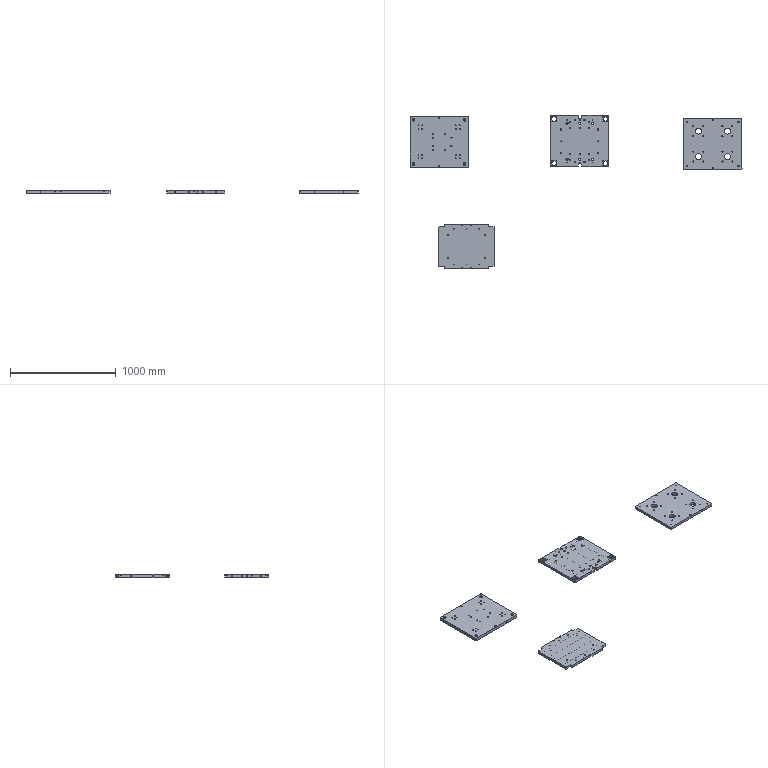NC program | Mastercam | posted with a generic post | part box 3140 x 1452 x 30 mm
Lines 1 to 1155 of 29880:
%
O0000()
(MATERIAL - ALUMINUM MM - 2024)
( T16 | 16 FEM | H16 | XY STOCK TO LEAVE - .1 | Z STOCK TO LEAVE - .05 )
( T12 | 12 FEM | H12 | XY STOCK TO LEAVE - 0. | Z STOCK TO LEAVE - .05 )
( T7 | 4 CHM | H7 )
( T1 | 11 DR | H1 | XY STOCK TO LEAVE - 0. | Z STOCK TO LEAVE - .15 )
( T3 | 10.5 DR | H3 )
( T6 | 6 FEM | H6 | XY STOCK TO LEAVE - .05 | Z STOCK TO LEAVE - .15 )
( T15 | 5.2 DR | H15 )
N100 G21
N110 G0 G17 G40 G49 G80 G90
( ? )
N120 T16 M6
N130 G0 G90 G54 X283.1 Y252.5 A0. S6000 M3
N140 G43 H16 Z50. M8
N150 Z1.2
N160 G1 Z-.293 F600.
N170 Y237.5 F4000.
N180 Y-237.5
N190 Y-252.5
N200 Z-.786 F600.
N210 Y-237.5 F4000.
N220 Y237.5
N230 Y252.5
N240 Z-1.279 F600.
N250 Y237.5 F4000.
N260 Y-237.5
N270 Y-252.5
N280 Z-1.773 F600.
N290 Y-237.5 F4000.
N300 Y237.5
N310 Y252.5
N320 Z-2.266 F600.
N330 Y237.5 F4000.
N340 Y-237.5
N350 Y-252.5
N360 Z-2.759 F600.
N370 Y-237.5 F4000.
N380 Y237.5
N390 Y252.5
N400 Z-3.252 F600.
N410 Y237.5 F4000.
N420 Y-237.5
N430 Y-252.5
N440 Z-3.745 F600.
N450 Y-237.5 F4000.
N460 Y237.5
N470 Y252.5
N480 Z-4.238 F600.
N490 Y237.5 F4000.
N500 Y-237.5
N510 Y-252.5
N520 Z-4.731 F600.
N530 Y-237.5 F4000.
N540 Y237.5
N550 Y252.5
N560 Z-5.225 F600.
N570 Y237.5 F4000.
N580 Y-237.5
N590 Y-252.5
N600 Z-5.718 F600.
N610 Y-237.5 F4000.
N620 Y237.5
N630 Y252.5
N640 Z-6.211 F600.
N650 Y237.5 F4000.
N660 Y-237.5
N670 Y-252.5
N680 Z-6.704 F600.
N690 Y-237.5 F4000.
N700 Y237.5
N710 Y252.5
N720 Z-7.197 F600.
N730 Y237.5 F4000.
N740 Y-237.5
N750 Y-252.5
N760 Z-7.69 F600.
N770 Y-237.5 F4000.
N780 Y237.5
N790 Y252.5
N800 Z-8.183 F600.
N810 Y237.5 F4000.
N820 Y-237.5
N830 Y-252.5
N840 Z-8.676 F600.
N850 Y-237.5 F4000.
N860 Y237.5
N870 Y252.5
N880 Z-9.17 F600.
N890 Y237.5 F4000.
N900 Y-237.5
N910 Y-252.5
N920 Z-9.663 F600.
N930 Y-237.5 F4000.
N940 Y237.5
N950 Y252.5
N960 Z-10.156 F600.
N970 Y237.5 F4000.
N980 Y-237.5
N990 Y-252.5
N1000 Z-10.649 F600.
N1010 Y-237.5 F4000.
N1020 Y237.5
N1030 Y252.5
N1040 Z-11.142 F600.
N1050 Y237.5 F4000.
N1060 Y-237.5
N1070 Y-252.5
N1080 Z-11.635 F600.
N1090 Y-237.5 F4000.
N1100 Y237.5
N1110 Y252.5
N1120 Z-12.128 F600.
N1130 Y237.5 F4000.
N1140 Y-237.5
N1150 Y-252.5
N1160 Z-12.622 F600.
N1170 Y-237.5 F4000.
N1180 Y237.5
N1190 Y252.5
N1200 Z-13.115 F600.
N1210 Y237.5 F4000.
N1220 Y-237.5
N1230 Y-252.5
N1240 Z-13.608 F600.
N1250 Y-237.5 F4000.
N1260 Y237.5
N1270 Y252.5
N1280 Z-14.101 F600.
N1290 Y237.5 F4000.
N1300 Y-237.5
N1310 Y-252.5
N1320 Z-14.594 F600.
N1330 Y-237.5 F4000.
N1340 Y237.5
N1350 Y252.5
N1360 Z-15.087 F600.
N1370 Y237.5 F4000.
N1380 Y-237.5
N1390 Y-252.5
N1400 Z-15.58 F600.
N1410 Y-237.5 F4000.
N1420 Y237.5
N1430 Y252.5
N1440 Z-16.074 F600.
N1450 Y237.5 F4000.
N1460 Y-237.5
N1470 Y-252.5
N1480 Z-16.567 F600.
N1490 Y-237.5 F4000.
N1500 Y237.5
N1510 Y252.5
N1520 Z-17.06 F600.
N1530 Y237.5 F4000.
N1540 Y-237.5
N1550 Y-252.5
N1560 Z-17.553 F600.
N1570 Y-237.5 F4000.
N1580 Y237.5
N1590 Y252.5
N1600 Z-18.046 F600.
N1610 Y237.5 F4000.
N1620 Y-237.5
N1630 Y-252.5
N1640 Z-18.539 F600.
N1650 Y-237.5 F4000.
N1660 Y237.5
N1670 Y252.5
N1680 Z-19.032 F600.
N1690 Y237.5 F4000.
N1700 Y-237.5
N1710 Y-252.5
N1720 Z-19.525 F600.
N1730 Y-237.5 F4000.
N1740 Y237.5
N1750 Y252.5
N1760 Z-20.019 F600.
N1770 Y237.5 F4000.
N1780 Y-237.5
N1790 Y-252.5
N1800 Z-20.512 F600.
N1810 Y-237.5 F4000.
N1820 Y237.5
N1830 Y252.5
N1840 Z-21.005 F600.
N1850 Y237.5 F4000.
N1860 Y-237.5
N1870 Y-252.5
N1880 Z-21.498 F600.
N1890 Y-237.5 F4000.
N1900 Y237.5
N1910 Y252.5
N1920 Z-21.991 F600.
N1930 Y237.5 F4000.
N1940 Y-237.5
N1950 Y-252.5
N1960 Z-22.484 F600.
N1970 Y-237.5 F4000.
N1980 Y237.5
N1990 Y252.5
N2000 Z-22.977 F600.
N2010 Y237.5 F4000.
N2020 Y-237.5
N2030 Y-252.5
N2040 Z-23.471 F600.
N2050 Y-237.5 F4000.
N2060 Y237.5
N2070 Y252.5
N2080 Z-23.964 F600.
N2090 Y237.5 F4000.
N2100 Y-237.5
N2110 Y-252.5
N2120 Z-24.457 F600.
N2130 Y-237.5 F4000.
N2140 Y237.5
N2150 Y252.5
N2160 Z-24.95 F600.
N2170 Y237.5 F4000.
N2180 Y-237.5
N2190 Y-252.5
N2200 G0 Z50.
N2210 X-283.1
N2220 Z1.2
N2230 G1 Z-.293 F600.
N2240 Y-237.5 F4000.
N2250 Y237.5
N2260 Y252.5
N2270 Z-.786 F600.
N2280 Y237.5 F4000.
N2290 Y-237.5
N2300 Y-252.5
N2310 Z-1.279 F600.
N2320 Y-237.5 F4000.
N2330 Y237.5
N2340 Y252.5
N2350 Z-1.773 F600.
N2360 Y237.5 F4000.
N2370 Y-237.5
N2380 Y-252.5
N2390 Z-2.266 F600.
N2400 Y-237.5 F4000.
N2410 Y237.5
N2420 Y252.5
N2430 Z-2.759 F600.
N2440 Y237.5 F4000.
N2450 Y-237.5
N2460 Y-252.5
N2470 Z-3.252 F600.
N2480 Y-237.5 F4000.
N2490 Y237.5
N2500 Y252.5
N2510 Z-3.745 F600.
N2520 Y237.5 F4000.
N2530 Y-237.5
N2540 Y-252.5
N2550 Z-4.238 F600.
N2560 Y-237.5 F4000.
N2570 Y237.5
N2580 Y252.5
N2590 Z-4.731 F600.
N2600 Y237.5 F4000.
N2610 Y-237.5
N2620 Y-252.5
N2630 Z-5.225 F600.
N2640 Y-237.5 F4000.
N2650 Y237.5
N2660 Y252.5
N2670 Z-5.718 F600.
N2680 Y237.5 F4000.
N2690 Y-237.5
N2700 Y-252.5
N2710 Z-6.211 F600.
N2720 Y-237.5 F4000.
N2730 Y237.5
N2740 Y252.5
N2750 Z-6.704 F600.
N2760 Y237.5 F4000.
N2770 Y-237.5
N2780 Y-252.5
N2790 Z-7.197 F600.
N2800 Y-237.5 F4000.
N2810 Y237.5
N2820 Y252.5
N2830 Z-7.69 F600.
N2840 Y237.5 F4000.
N2850 Y-237.5
N2860 Y-252.5
N2870 Z-8.183 F600.
N2880 Y-237.5 F4000.
N2890 Y237.5
N2900 Y252.5
N2910 Z-8.676 F600.
N2920 Y237.5 F4000.
N2930 Y-237.5
N2940 Y-252.5
N2950 Z-9.17 F600.
N2960 Y-237.5 F4000.
N2970 Y237.5
N2980 Y252.5
N2990 Z-9.663 F600.
N3000 Y237.5 F4000.
N3010 Y-237.5
N3020 Y-252.5
N3030 Z-10.156 F600.
N3040 Y-237.5 F4000.
N3050 Y237.5
N3060 Y252.5
N3070 Z-10.649 F600.
N3080 Y237.5 F4000.
N3090 Y-237.5
N3100 Y-252.5
N3110 Z-11.142 F600.
N3120 Y-237.5 F4000.
N3130 Y237.5
N3140 Y252.5
N3150 Z-11.635 F600.
N3160 Y237.5 F4000.
N3170 Y-237.5
N3180 Y-252.5
N3190 Z-12.128 F600.
N3200 Y-237.5 F4000.
N3210 Y237.5
N3220 Y252.5
N3230 Z-12.622 F600.
N3240 Y237.5 F4000.
N3250 Y-237.5
N3260 Y-252.5
N3270 Z-13.115 F600.
N3280 Y-237.5 F4000.
N3290 Y237.5
N3300 Y252.5
N3310 Z-13.608 F600.
N3320 Y237.5 F4000.
N3330 Y-237.5
N3340 Y-252.5
N3350 Z-14.101 F600.
N3360 Y-237.5 F4000.
N3370 Y237.5
N3380 Y252.5
N3390 Z-14.594 F600.
N3400 Y237.5 F4000.
N3410 Y-237.5
N3420 Y-252.5
N3430 Z-15.087 F600.
N3440 Y-237.5 F4000.
N3450 Y237.5
N3460 Y252.5
N3470 Z-15.58 F600.
N3480 Y237.5 F4000.
N3490 Y-237.5
N3500 Y-252.5
N3510 Z-16.074 F600.
N3520 Y-237.5 F4000.
N3530 Y237.5
N3540 Y252.5
N3550 Z-16.567 F600.
N3560 Y237.5 F4000.
N3570 Y-237.5
N3580 Y-252.5
N3590 Z-17.06 F600.
N3600 Y-237.5 F4000.
N3610 Y237.5
N3620 Y252.5
N3630 Z-17.553 F600.
N3640 Y237.5 F4000.
N3650 Y-237.5
N3660 Y-252.5
N3670 Z-18.046 F600.
N3680 Y-237.5 F4000.
N3690 Y237.5
N3700 Y252.5
N3710 Z-18.539 F600.
N3720 Y237.5 F4000.
N3730 Y-237.5
N3740 Y-252.5
N3750 Z-19.032 F600.
N3760 Y-237.5 F4000.
N3770 Y237.5
N3780 Y252.5
N3790 Z-19.525 F600.
N3800 Y237.5 F4000.
N3810 Y-237.5
N3820 Y-252.5
N3830 Z-20.019 F600.
N3840 Y-237.5 F4000.
N3850 Y237.5
N3860 Y252.5
N3870 Z-20.512 F600.
N3880 Y237.5 F4000.
N3890 Y-237.5
N3900 Y-252.5
N3910 Z-21.005 F600.
N3920 Y-237.5 F4000.
N3930 Y237.5
N3940 Y252.5
N3950 Z-21.498 F600.
N3960 Y237.5 F4000.
N3970 Y-237.5
N3980 Y-252.5
N3990 Z-21.991 F600.
N4000 Y-237.5 F4000.
N4010 Y237.5
N4020 Y252.5
N4030 Z-22.484 F600.
N4040 Y237.5 F4000.
N4050 Y-237.5
N4060 Y-252.5
N4070 Z-22.977 F600.
N4080 Y-237.5 F4000.
N4090 Y237.5
N4100 Y252.5
N4110 Z-23.471 F600.
N4120 Y237.5 F4000.
N4130 Y-237.5
N4140 Y-252.5
N4150 Z-23.964 F600.
N4160 Y-237.5 F4000.
N4170 Y237.5
N4180 Y252.5
N4190 Z-24.457 F600.
N4200 Y237.5 F4000.
N4210 Y-237.5
N4220 Y-252.5
N4230 Z-24.95 F600.
N4240 Y-237.5 F4000.
N4250 Y237.5
N4260 Y252.5
N4270 G0 Z50.
N4280 M5
N4290 G91 G28 Z0. M9
N4300 A0.
N4310 M01
N4320 T12 M6
N4330 G0 G90 G17 G54 X281. Y249.5 A0. S7000 M3
N4340 G43 H12 Z50. M8
N4350 Z1.2
N4360 G1 Z-12.375 F600.
N4370 Y237.5 F1000.
N4380 Y-237.5
N4390 Y-249.5
N4400 G0 Z50.
N4410 Y249.5
N4420 Z-11.375
N4430 G1 Z-24.95 F600.
N4440 Y237.5 F1000.
N4450 Y-237.5
N4460 Y-249.5
N4470 G0 Z50.
N4480 X-281.
N4490 Z1.2
N4500 G1 Z-12.375 F600.
N4510 Y-237.5 F1000.
N4520 Y237.5
N4530 Y249.5
N4540 G0 Z50.
N4550 Y-249.5
N4560 Z-11.375
N4570 G1 Z-24.95 F600.
N4580 Y-237.5 F1000.
N4590 Y237.5
N4600 Y249.5
N4610 G0 Z50.
N4620 M5
N4630 G91 G28 Z0. M9
N4640 A0.
N4650 M01
N4660 T7 M6
N4670 G0 G90 G17 G54 X275.65 Y243.5 A0. S7000 M3
N4680 G43 H7 Z50. M8
N4690 Z1.2
N4700 G1 Z-.75 F600.
N4710 Y237.5 F1000.
N4720 Y-237.5
N4730 Y-243.5
N4740 G0 Z50.
N4750 X-275.65
N4760 Z1.2
N4770 G1 Z-.75 F600.
N4780 Y-237.5 F1000.
N4790 Y237.5
N4800 Y243.5
N4810 G0 Z50.
N4820 M5
N4830 G91 G28 Z0. M9
N4840 A0.
N4850 M01
( ?X )
M00
N4860 T16 M6
N4870 G0 G90 G17 G54 X286.3 Y-235.9 A0. S6000 M3
N4880 G43 H16 Z50. M8
N4890 Z1.2
N4900 G1 Z-.499 F600.
N4910 X284.7 F4000.
N4920 G3 X283.1 Y-237.5 I0. J-1.6
N4930 G2 X270. Y-250.6 I-13.1 J0.
N4940 G1 X-270.
N4950 G2 X-283.1 Y-237.5 I0. J13.1
N4960 G3 X-284.7 Y-235.9 I-1.6 J0.
N4970 G1 X-286.3
N4980 Z-1.197 F600.
N4990 X-284.7 F4000.
N5000 G2 X-283.1 Y-237.5 I0. J-1.6
N5010 G3 X-270. Y-250.6 I13.1 J0.
N5020 G1 X270.
N5030 G3 X283.1 Y-237.5 I0. J13.1
N5040 G2 X284.7 Y-235.9 I1.6 J0.
N5050 G1 X286.3
N5060 Z-1.896 F600.
N5070 X284.7 F4000.
N5080 G3 X283.1 Y-237.5 I0. J-1.6
N5090 G2 X270. Y-250.6 I-13.1 J0.
N5100 G1 X-270.
N5110 G2 X-283.1 Y-237.5 I0. J13.1
N5120 G3 X-284.7 Y-235.9 I-1.6 J0.
N5130 G1 X-286.3
N5140 Z-2.594 F600.
N5150 X-284.7 F4000.
N5160 G2 X-283.1 Y-237.5 I0. J-1.6
N5170 G3 X-270. Y-250.6 I13.1 J0.
N5180 G1 X270.
N5190 G3 X283.1 Y-237.5 I0. J13.1
N5200 G2 X284.7 Y-235.9 I1.6 J0.
N5210 G1 X286.3
N5220 Z-3.293 F600.
N5230 X284.7 F4000.
N5240 G3 X283.1 Y-237.5 I0. J-1.6
N5250 G2 X270. Y-250.6 I-13.1 J0.
N5260 G1 X-270.
N5270 G2 X-283.1 Y-237.5 I0. J13.1
N5280 G3 X-284.7 Y-235.9 I-1.6 J0.
N5290 G1 X-286.3
N5300 Z-3.992 F600.
N5310 X-284.7 F4000.
N5320 G2 X-283.1 Y-237.5 I0. J-1.6
N5330 G3 X-270. Y-250.6 I13.1 J0.
N5340 G1 X270.
N5350 G3 X283.1 Y-237.5 I0. J13.1
N5360 G2 X284.7 Y-235.9 I1.6 J0.
N5370 G1 X286.3
N5380 Z-4.69 F600.
N5390 X284.7 F4000.
N5400 G3 X283.1 Y-237.5 I0. J-1.6
N5410 G2 X270. Y-250.6 I-13.1 J0.
N5420 G1 X-270.
N5430 G2 X-283.1 Y-237.5 I0. J13.1
N5440 G3 X-284.7 Y-235.9 I-1.6 J0.
N5450 G1 X-286.3
N5460 Z-5.389 F600.
N5470 X-284.7 F4000.
N5480 G2 X-283.1 Y-237.5 I0. J-1.6
N5490 G3 X-270. Y-250.6 I13.1 J0.
N5500 G1 X270.
N5510 G3 X283.1 Y-237.5 I0. J13.1
N5520 G2 X284.7 Y-235.9 I1.6 J0.
N5530 G1 X286.3
N5540 Z-6.088 F600.
N5550 X284.7 F4000.
N5560 G3 X283.1 Y-237.5 I0. J-1.6
N5570 G2 X270. Y-250.6 I-13.1 J0.
N5580 G1 X-270.
N5590 G2 X-283.1 Y-237.5 I0. J13.1
N5600 G3 X-284.7 Y-235.9 I-1.6 J0.
N5610 G1 X-286.3
N5620 Z-6.786 F600.
N5630 X-284.7 F4000.
N5640 G2 X-283.1 Y-237.5 I0. J-1.6
N5650 G3 X-270. Y-250.6 I13.1 J0.
N5660 G1 X270.
N5670 G3 X283.1 Y-237.5 I0. J13.1
N5680 G2 X284.7 Y-235.9 I1.6 J0.
N5690 G1 X286.3
N5700 Z-7.485 F600.
N5710 X284.7 F4000.
N5720 G3 X283.1 Y-237.5 I0. J-1.6
N5730 G2 X270. Y-250.6 I-13.1 J0.
N5740 G1 X-270.
N5750 G2 X-283.1 Y-237.5 I0. J13.1
N5760 G3 X-284.7 Y-235.9 I-1.6 J0.
N5770 G1 X-286.3
N5780 Z-8.183 F600.
N5790 X-284.7 F4000.
N5800 G2 X-283.1 Y-237.5 I0. J-1.6
N5810 G3 X-270. Y-250.6 I13.1 J0.
N5820 G1 X270.
N5830 G3 X283.1 Y-237.5 I0. J13.1
N5840 G2 X284.7 Y-235.9 I1.6 J0.
N5850 G1 X286.3
N5860 Z-8.882 F600.
N5870 X284.7 F4000.
N5880 G3 X283.1 Y-237.5 I0. J-1.6
N5890 G2 X270. Y-250.6 I-13.1 J0.
N5900 G1 X-270.
N5910 G2 X-283.1 Y-237.5 I0. J13.1
N5920 G3 X-284.7 Y-235.9 I-1.6 J0.
N5930 G1 X-286.3
N5940 Z-9.581 F600.
N5950 X-284.7 F4000.
N5960 G2 X-283.1 Y-237.5 I0. J-1.6
N5970 G3 X-270. Y-250.6 I13.1 J0.
N5980 G1 X270.
N5990 G3 X283.1 Y-237.5 I0. J13.1
N6000 G2 X284.7 Y-235.9 I1.6 J0.
N6010 G1 X286.3
N6020 Z-10.279 F600.
N6030 X284.7 F4000.
N6040 G3 X283.1 Y-237.5 I0. J-1.6
N6050 G2 X270. Y-250.6 I-13.1 J0.
N6060 G1 X-270.
N6070 G2 X-283.1 Y-237.5 I0. J13.1
N6080 G3 X-284.7 Y-235.9 I-1.6 J0.
N6090 G1 X-286.3
N6100 Z-10.978 F600.
N6110 X-284.7 F4000.
N6120 G2 X-283.1 Y-237.5 I0. J-1.6
N6130 G3 X-270. Y-250.6 I13.1 J0.
N6140 G1 X270.
N6150 G3 X283.1 Y-237.5 I0. J13.1
N6160 G2 X284.7 Y-235.9 I1.6 J0.
N6170 G1 X286.3
N6180 Z-11.676 F600.
N6190 X284.7 F4000.
N6200 G3 X283.1 Y-237.5 I0. J-1.6
N6210 G2 X270. Y-250.6 I-13.1 J0.
N6220 G1 X-270.
N6230 G2 X-283.1 Y-237.5 I0. J13.1
N6240 G3 X-284.7 Y-235.9 I-1.6 J0.
N6250 G1 X-286.3
N6260 Z-12.375 F600.
N6270 X-284.7 F4000.
N6280 G2 X-283.1 Y-237.5 I0. J-1.6
N6290 G3 X-270. Y-250.6 I13.1 J0.
N6300 G1 X270.
N6310 G3 X283.1 Y-237.5 I0. J13.1
N6320 G2 X284.7 Y-235.9 I1.6 J0.
N6330 G1 X286.3
N6340 Z-13.074 F600.
N6350 X284.7 F4000.
N6360 G3 X283.1 Y-237.5 I0. J-1.6
N6370 G2 X270. Y-250.6 I-13.1 J0.
N6380 G1 X-270.
N6390 G2 X-283.1 Y-237.5 I0. J13.1
N6400 G3 X-284.7 Y-235.9 I-1.6 J0.
N6410 G1 X-286.3
N6420 Z-13.772 F600.
N6430 X-284.7 F4000.
N6440 G2 X-283.1 Y-237.5 I0. J-1.6
N6450 G3 X-270. Y-250.6 I13.1 J0.
N6460 G1 X270.
N6470 G3 X283.1 Y-237.5 I0. J13.1
N6480 G2 X284.7 Y-235.9 I1.6 J0.
N6490 G1 X286.3
N6500 Z-14.471 F600.
N6510 X284.7 F4000.
N6520 G3 X283.1 Y-237.5 I0. J-1.6
N6530 G2 X270. Y-250.6 I-13.1 J0.
N6540 G1 X-270.
N6550 G2 X-283.1 Y-237.5 I0. J13.1
N6560 G3 X-284.7 Y-235.9 I-1.6 J0.
N6570 G1 X-286.3
N6580 Z-15.169 F600.
N6590 X-284.7 F4000.
N6600 G2 X-283.1 Y-237.5 I0. J-1.6
N6610 G3 X-270. Y-250.6 I13.1 J0.
N6620 G1 X270.
N6630 G3 X283.1 Y-237.5 I0. J13.1
N6640 G2 X284.7 Y-235.9 I1.6 J0.
N6650 G1 X286.3
N6660 Z-15.868 F600.
N6670 X284.7 F4000.
N6680 G3 X283.1 Y-237.5 I0. J-1.6
N6690 G2 X270. Y-250.6 I-13.1 J0.
N6700 G1 X-270.
N6710 G2 X-283.1 Y-237.5 I0. J13.1
N6720 G3 X-284.7 Y-235.9 I-1.6 J0.
N6730 G1 X-286.3
N6740 Z-16.567 F600.
N6750 X-284.7 F4000.
N6760 G2 X-283.1 Y-237.5 I0. J-1.6
N6770 G3 X-270. Y-250.6 I13.1 J0.
N6780 G1 X270.
N6790 G3 X283.1 Y-237.5 I0. J13.1
N6800 G2 X284.7 Y-235.9 I1.6 J0.
N6810 G1 X286.3
N6820 Z-17.265 F600.
N6830 X284.7 F4000.
N6840 G3 X283.1 Y-237.5 I0. J-1.6
N6850 G2 X270. Y-250.6 I-13.1 J0.
N6860 G1 X-270.
N6870 G2 X-283.1 Y-237.5 I0. J13.1
N6880 G3 X-284.7 Y-235.9 I-1.6 J0.
N6890 G1 X-286.3
N6900 Z-17.964 F600.
N6910 X-284.7 F4000.
N6920 G2 X-283.1 Y-237.5 I0. J-1.6
N6930 G3 X-270. Y-250.6 I13.1 J0.
N6940 G1 X270.
N6950 G3 X283.1 Y-237.5 I0. J13.1
N6960 G2 X284.7 Y-235.9 I1.6 J0.
N6970 G1 X286.3
N6980 Z-18.663 F600.
N6990 X284.7 F4000.
N7000 G3 X283.1 Y-237.5 I0. J-1.6
N7010 G2 X270. Y-250.6 I-13.1 J0.
N7020 G1 X-270.
N7030 G2 X-283.1 Y-237.5 I0. J13.1
N7040 G3 X-284.7 Y-235.9 I-1.6 J0.
N7050 G1 X-286.3
N7060 Z-19.361 F600.
N7070 X-284.7 F4000.
N7080 G2 X-283.1 Y-237.5 I0. J-1.6
N7090 G3 X-270. Y-250.6 I13.1 J0.
N7100 G1 X270.
N7110 G3 X283.1 Y-237.5 I0. J13.1
N7120 G2 X284.7 Y-235.9 I1.6 J0.
N7130 G1 X286.3
N7140 Z-20.06 F600.
N7150 X284.7 F4000.
N7160 G3 X283.1 Y-237.5 I0. J-1.6
N7170 G2 X270. Y-250.6 I-13.1 J0.
N7180 G1 X-270.
N7190 G2 X-283.1 Y-237.5 I0. J13.1
N7200 G3 X-284.7 Y-235.9 I-1.6 J0.
N7210 G1 X-286.3
N7220 Z-20.758 F600.
N7230 X-284.7 F4000.
N7240 G2 X-283.1 Y-237.5 I0. J-1.6
N7250 G3 X-270. Y-250.6 I13.1 J0.
N7260 G1 X270.
N7270 G3 X283.1 Y-237.5 I0. J13.1
N7280 G2 X284.7 Y-235.9 I1.6 J0.
N7290 G1 X286.3
N7300 Z-21.457 F600.
N7310 X284.7 F4000.
N7320 G3 X283.1 Y-237.5 I0. J-1.6
N7330 G2 X270. Y-250.6 I-13.1 J0.
N7340 G1 X-270.
N7350 G2 X-283.1 Y-237.5 I0. J13.1
N7360 G3 X-284.7 Y-235.9 I-1.6 J0.
N7370 G1 X-286.3
N7380 Z-22.156 F600.
N7390 X-284.7 F4000.
N7400 G2 X-283.1 Y-237.5 I0. J-1.6
N7410 G3 X-270. Y-250.6 I13.1 J0.
N7420 G1 X270.
N7430 G3 X283.1 Y-237.5 I0. J13.1
N7440 G2 X284.7 Y-235.9 I1.6 J0.
N7450 G1 X286.3
N7460 Z-22.854 F600.
N7470 X284.7 F4000.
N7480 G3 X283.1 Y-237.5 I0. J-1.6
N7490 G2 X270. Y-250.6 I-13.1 J0.
N7500 G1 X-270.
N7510 G2 X-283.1 Y-237.5 I0. J13.1
N7520 G3 X-284.7 Y-235.9 I-1.6 J0.
N7530 G1 X-286.3
N7540 Z-23.553 F600.
N7550 X-284.7 F4000.
N7560 G2 X-283.1 Y-237.5 I0. J-1.6
N7570 G3 X-270. Y-250.6 I13.1 J0.
N7580 G1 X270.
N7590 G3 X283.1 Y-237.5 I0. J13.1
N7600 G2 X284.7 Y-235.9 I1.6 J0.
N7610 G1 X286.3
N7620 Z-24.251 F600.
N7630 X284.7 F4000.
N7640 G3 X283.1 Y-237.5 I0. J-1.6
N7650 G2 X270. Y-250.6 I-13.1 J0.
N7660 G1 X-270.
N7670 G2 X-283.1 Y-237.5 I0. J13.1
N7680 G3 X-284.7 Y-235.9 I-1.6 J0.
N7690 G1 X-286.3
N7700 Z-24.95 F600.
N7710 X-284.7 F4000.
N7720 G2 X-283.1 Y-237.5 I0. J-1.6
N7730 G3 X-270. Y-250.6 I13.1 J0.
N7740 G1 X270.
N7750 G3 X283.1 Y-237.5 I0. J13.1
N7760 G2 X284.7 Y-235.9 I1.6 J0.
N7770 G1 X286.3
N7780 G0 Z50.
N7790 X-286.3 Y235.9
N7800 Z1.2
N7810 G1 Z-.499 F600.
N7820 X-284.7 F4000.
N7830 G3 X-283.1 Y237.5 I0. J1.6
N7840 G2 X-270. Y250.6 I13.1 J0.
N7850 G1 X270.
N7860 G2 X283.1 Y237.5 I0. J-13.1
N7870 G3 X284.7 Y235.9 I1.6 J0.
N7880 G1 X286.3
N7890 Z-1.197 F600.
N7900 X284.7 F4000.
N7910 G2 X283.1 Y237.5 I0. J1.6
N7920 G3 X270. Y250.6 I-13.1 J0.
N7930 G1 X-270.
N7940 G3 X-283.1 Y237.5 I0. J-13.1
N7950 G2 X-284.7 Y235.9 I-1.6 J0.
N7960 G1 X-286.3
N7970 Z-1.896 F600.
N7980 X-284.7 F4000.
N7990 G3 X-283.1 Y237.5 I0. J1.6
N8000 G2 X-270. Y250.6 I13.1 J0.
N8010 G1 X270.
N8020 G2 X283.1 Y237.5 I0. J-13.1
N8030 G3 X284.7 Y235.9 I1.6 J0.
N8040 G1 X286.3
N8050 Z-2.594 F600.
N8060 X284.7 F4000.
N8070 G2 X283.1 Y237.5 I0. J1.6
N8080 G3 X270. Y250.6 I-13.1 J0.
N8090 G1 X-270.
N8100 G3 X-283.1 Y237.5 I0. J-13.1
N8110 G2 X-284.7 Y235.9 I-1.6 J0.
N8120 G1 X-286.3
N8130 Z-3.293 F600.
N8140 X-284.7 F4000.
N8150 G3 X-283.1 Y237.5 I0. J1.6
N8160 G2 X-270. Y250.6 I13.1 J0.
N8170 G1 X270.
N8180 G2 X283.1 Y237.5 I0. J-13.1
N8190 G3 X284.7 Y235.9 I1.6 J0.
N8200 G1 X286.3
N8210 Z-3.992 F600.
N8220 X284.7 F4000.
N8230 G2 X283.1 Y237.5 I0. J1.6
N8240 G3 X270. Y250.6 I-13.1 J0.
N8250 G1 X-270.
N8260 G3 X-283.1 Y237.5 I0. J-13.1
N8270 G2 X-284.7 Y235.9 I-1.6 J0.
N8280 G1 X-286.3
N8290 Z-4.69 F600.
N8300 X-284.7 F4000.
N8310 G3 X-283.1 Y237.5 I0. J1.6
N8320 G2 X-270. Y250.6 I13.1 J0.
N8330 G1 X270.
N8340 G2 X283.1 Y237.5 I0. J-13.1
N8350 G3 X284.7 Y235.9 I1.6 J0.
N8360 G1 X286.3
N8370 Z-5.389 F600.
N8380 X284.7 F4000.
N8390 G2 X283.1 Y237.5 I0. J1.6
N8400 G3 X270. Y250.6 I-13.1 J0.
N8410 G1 X-270.
N8420 G3 X-283.1 Y237.5 I0. J-13.1
N8430 G2 X-284.7 Y235.9 I-1.6 J0.
N8440 G1 X-286.3
N8450 Z-6.088 F600.
N8460 X-284.7 F4000.
N8470 G3 X-283.1 Y237.5 I0. J1.6
N8480 G2 X-270. Y250.6 I13.1 J0.
N8490 G1 X270.
N8500 G2 X283.1 Y237.5 I0. J-13.1
N8510 G3 X284.7 Y235.9 I1.6 J0.
N8520 G1 X286.3
N8530 Z-6.786 F600.
N8540 X284.7 F4000.
N8550 G2 X283.1 Y237.5 I0. J1.6
N8560 G3 X270. Y250.6 I-13.1 J0.
N8570 G1 X-270.
N8580 G3 X-283.1 Y237.5 I0. J-13.1
N8590 G2 X-284.7 Y235.9 I-1.6 J0.
N8600 G1 X-286.3
N8610 Z-7.485 F600.
N8620 X-284.7 F4000.
N8630 G3 X-283.1 Y237.5 I0. J1.6
N8640 G2 X-270. Y250.6 I13.1 J0.
N8650 G1 X270.
N8660 G2 X283.1 Y237.5 I0. J-13.1
N8670 G3 X284.7 Y235.9 I1.6 J0.
N8680 G1 X286.3
N8690 Z-8.183 F600.
N8700 X284.7 F4000.
N8710 G2 X283.1 Y237.5 I0. J1.6
N8720 G3 X270. Y250.6 I-13.1 J0.
N8730 G1 X-270.
N8740 G3 X-283.1 Y237.5 I0. J-13.1
N8750 G2 X-284.7 Y235.9 I-1.6 J0.
N8760 G1 X-286.3
N8770 Z-8.882 F600.
N8780 X-284.7 F4000.
N8790 G3 X-283.1 Y237.5 I0. J1.6
N8800 G2 X-270. Y250.6 I13.1 J0.
N8810 G1 X270.
N8820 G2 X283.1 Y237.5 I0. J-13.1
N8830 G3 X284.7 Y235.9 I1.6 J0.
N8840 G1 X286.3
N8850 Z-9.581 F600.
N8860 X284.7 F4000.
N8870 G2 X283.1 Y237.5 I0. J1.6
N8880 G3 X270. Y250.6 I-13.1 J0.
N8890 G1 X-270.
N8900 G3 X-283.1 Y237.5 I0. J-13.1
N8910 G2 X-284.7 Y235.9 I-1.6 J0.
N8920 G1 X-286.3
N8930 Z-10.279 F600.
N8940 X-284.7 F4000.
N8950 G3 X-283.1 Y237.5 I0. J1.6
N8960 G2 X-270. Y250.6 I13.1 J0.
N8970 G1 X270.
N8980 G2 X283.1 Y237.5 I0. J-13.1
N8990 G3 X284.7 Y235.9 I1.6 J0.
N9000 G1 X286.3
N9010 Z-10.978 F600.
N9020 X284.7 F4000.
N9030 G2 X283.1 Y237.5 I0. J1.6
N9040 G3 X270. Y250.6 I-13.1 J0.
N9050 G1 X-270.
N9060 G3 X-283.1 Y237.5 I0. J-13.1
N9070 G2 X-284.7 Y235.9 I-1.6 J0.
N9080 G1 X-286.3
N9090 Z-11.676 F600.
N9100 X-284.7 F4000.
N9110 G3 X-283.1 Y237.5 I0. J1.6
N9120 G2 X-270. Y250.6 I13.1 J0.
N9130 G1 X270.
N9140 G2 X283.1 Y237.5 I0. J-13.1
N9150 G3 X284.7 Y235.9 I1.6 J0.
N9160 G1 X286.3
N9170 Z-12.375 F600.
N9180 X284.7 F4000.
N9190 G2 X283.1 Y237.5 I0. J1.6
N9200 G3 X270. Y250.6 I-13.1 J0.
N9210 G1 X-270.
N9220 G3 X-283.1 Y237.5 I0. J-13.1
N9230 G2 X-284.7 Y235.9 I-1.6 J0.
N9240 G1 X-286.3
N9250 Z-13.074 F600.
N9260 X-284.7 F4000.
N9270 G3 X-283.1 Y237.5 I0. J1.6
N9280 G2 X-270. Y250.6 I13.1 J0.
N9290 G1 X270.
N9300 G2 X283.1 Y237.5 I0. J-13.1
N9310 G3 X284.7 Y235.9 I1.6 J0.
N9320 G1 X286.3
N9330 Z-13.772 F600.
N9340 X284.7 F4000.
N9350 G2 X283.1 Y237.5 I0. J1.6
N9360 G3 X270. Y250.6 I-13.1 J0.
N9370 G1 X-270.
N9380 G3 X-283.1 Y237.5 I0. J-13.1
N9390 G2 X-284.7 Y235.9 I-1.6 J0.
N9400 G1 X-286.3
N9410 Z-14.471 F600.
N9420 X-284.7 F4000.
N9430 G3 X-283.1 Y237.5 I0. J1.6
N9440 G2 X-270. Y250.6 I13.1 J0.
N9450 G1 X270.
N9460 G2 X283.1 Y237.5 I0. J-13.1
N9470 G3 X284.7 Y235.9 I1.6 J0.
N9480 G1 X286.3
N9490 Z-15.169 F600.
N9500 X284.7 F4000.
N9510 G2 X283.1 Y237.5 I0. J1.6
N9520 G3 X270. Y250.6 I-13.1 J0.
N9530 G1 X-270.
N9540 G3 X-283.1 Y237.5 I0. J-13.1
N9550 G2 X-284.7 Y235.9 I-1.6 J0.
N9560 G1 X-286.3
N9570 Z-15.868 F600.
N9580 X-284.7 F4000.
N9590 G3 X-283.1 Y237.5 I0. J1.6
N9600 G2 X-270. Y250.6 I13.1 J0.
N9610 G1 X270.
N9620 G2 X283.1 Y237.5 I0. J-13.1
N9630 G3 X284.7 Y235.9 I1.6 J0.
N9640 G1 X286.3
N9650 Z-16.567 F600.
N9660 X284.7 F4000.
N9670 G2 X283.1 Y237.5 I0. J1.6
N9680 G3 X270. Y250.6 I-13.1 J0.
N9690 G1 X-270.
N9700 G3 X-283.1 Y237.5 I0. J-13.1
N9710 G2 X-284.7 Y235.9 I-1.6 J0.
N9720 G1 X-286.3
N9730 Z-17.265 F600.
N9740 X-284.7 F4000.
N9750 G3 X-283.1 Y237.5 I0. J1.6
N9760 G2 X-270. Y250.6 I13.1 J0.
N9770 G1 X270.
N9780 G2 X283.1 Y237.5 I0. J-13.1
N9790 G3 X284.7 Y235.9 I1.6 J0.
N9800 G1 X286.3
N9810 Z-17.964 F600.
N9820 X284.7 F4000.
N9830 G2 X283.1 Y237.5 I0. J1.6
N9840 G3 X270. Y250.6 I-13.1 J0.
N9850 G1 X-270.
N9860 G3 X-283.1 Y237.5 I0. J-13.1
N9870 G2 X-284.7 Y235.9 I-1.6 J0.
N9880 G1 X-286.3
N9890 Z-18.663 F600.
N9900 X-284.7 F4000.
N9910 G3 X-283.1 Y237.5 I0. J1.6
N9920 G2 X-270. Y250.6 I13.1 J0.
N9930 G1 X270.
N9940 G2 X283.1 Y237.5 I0. J-13.1
N9950 G3 X284.7 Y235.9 I1.6 J0.
N9960 G1 X286.3
N9970 Z-19.361 F600.
N9980 X284.7 F4000.
N9990 G2 X283.1 Y237.5 I0. J1.6
N100 G3 X270. Y250.6 I-13.1 J0.
N110 G1 X-270.
N120 G3 X-283.1 Y237.5 I0. J-13.1
N130 G2 X-284.7 Y235.9 I-1.6 J0.
N140 G1 X-286.3
N150 Z-20.06 F600.
N160 X-284.7 F4000.
N170 G3 X-283.1 Y237.5 I0. J1.6
N180 G2 X-270. Y250.6 I13.1 J0.
N190 G1 X270.
N200 G2 X283.1 Y237.5 I0. J-13.1
N210 G3 X284.7 Y235.9 I1.6 J0.
N220 G1 X286.3
N230 Z-20.758 F600.
N240 X284.7 F4000.
N250 G2 X283.1 Y237.5 I0. J1.6
N260 G3 X270. Y250.6 I-13.1 J0.
N270 G1 X-270.
N280 G3 X-283.1 Y237.5 I0. J-13.1
N290 G2 X-284.7 Y235.9 I-1.6 J0.
N300 G1 X-286.3
N310 Z-21.457 F600.
N320 X-284.7 F4000.
N330 G3 X-283.1 Y237.5 I0. J1.6
N340 G2 X-270. Y250.6 I13.1 J0.
N350 G1 X270.
N360 G2 X283.1 Y237.5 I0. J-13.1
N370 G3 X284.7 Y235.9 I1.6 J0.
N380 G1 X286.3
N390 Z-22.156 F600.
N400 X284.7 F4000.
N410 G2 X283.1 Y237.5 I0. J1.6
N420 G3 X270. Y250.6 I-13.1 J0.
N430 G1 X-270.
N440 G3 X-283.1 Y237.5 I0. J-13.1
N450 G2 X-284.7 Y235.9 I-1.6 J0.
N460 G1 X-286.3
N470 Z-22.854 F600.
N480 X-284.7 F4000.
N490 G3 X-283.1 Y237.5 I0. J1.6
N500 G2 X-270. Y250.6 I13.1 J0.
N510 G1 X270.
N520 G2 X283.1 Y237.5 I0. J-13.1
N530 G3 X284.7 Y235.9 I1.6 J0.
N540 G1 X286.3
N550 Z-23.553 F600.
N560 X284.7 F4000.
N570 G2 X283.1 Y237.5 I0. J1.6
N580 G3 X270. Y250.6 I-13.1 J0.
N590 G1 X-270.
N600 G3 X-283.1 Y237.5 I0. J-13.1
N610 G2 X-284.7 Y235.9 I-1.6 J0.
N620 G1 X-286.3
N630 Z-24.251 F600.
N640 X-284.7 F4000.
N650 G3 X-283.1 Y237.5 I0. J1.6
N660 G2 X-270. Y250.6 I13.1 J0.
N670 G1 X270.
N680 G2 X283.1 Y237.5 I0. J-13.1
N690 G3 X284.7 Y235.9 I1.6 J0.
N700 G1 X286.3
N710 Z-24.95 F600.
N720 X284.7 F4000.
N730 G2 X283.1 Y237.5 I0. J1.6
N740 G3 X270. Y250.6 I-13.1 J0.
N750 G1 X-270.
N760 G3 X-283.1 Y237.5 I0. J-13.1
N770 G2 X-284.7 Y235.9 I-1.6 J0.
N780 G1 X-286.3
N790 G0 Z50.
N800 M5
N810 G91 G28 Z0. M9
N820 A0.
N830 M01
N840 T12 M6
N850 G0 G90 G17 G54 X283.4 Y-236.3 A0. S6000 M3
N860 G43 H12 Z50. M8
N870 Z1.2
N880 G1 Z-12.375 F600.
N890 X282.2 F1000.
N900 G3 X281. Y-237.5 I0. J-1.2
N910 G2 X270. Y-248.5 I-11. J0.
N920 G1 X-270.
N930 G2 X-281. Y-237.5 I0. J11.
N940 G3 X-282.2 Y-236.3 I-1.2 J0.
N950 G1 X-283.4
N960 G0 Z50.
N970 X283.4
N980 Z-11.375
N990 G1 Z-24.95 F600.
N1000 X282.2 F1000.
N1010 G3 X281. Y-237.5 I0. J-1.2
N1020 G2 X270. Y-248.5 I-11. J0.
N1030 G1 X-270.
N1040 G2 X-281. Y-237.5 I0. J11.
N1050 G3 X-282.2 Y-236.3 I-1.2 J0.
N1060 G1 X-283.4
N1070 G0 Z50.
N1080 Y236.3
N1090 Z1.2
N1100 G1 Z-12.375 F600.
N1110 X-282.2 F1000.
N1120 G3 X-281. Y237.5 I0. J1.2
N1130 G2 X-270. Y248.5 I11. J0.
N1140 G1 X270.
N1150 G2 X281. Y237.5 I0. J-11.
N1160 G3 X282.2 Y236.3 I1.2 J0.
N1170 G1 X283.4
N1180 G0 Z50.
N1190 X-283.4
N1200 Z-11.375
N1210 G1 Z-24.95 F600.
N1220 X-282.2 F1000.
N1230 G3 X-281. Y237.5 I0. J1.2
N1240 G2 X-270. Y248.5 I11. J0.
N1250 G1 X270.
N1260 G2 X281. Y237.5 I0. J-11.
N1270 G3 X282.2 Y236.3 I1.2 J0.
N1280 G1 X283.4
N1290 G0 Z50.
N1300 M5
N1310 G91 G28 Z0. M9
N1320 A0.
N1330 M01
N1340 T7 M6
N1350 G0 G90 G17 G54 X276.45 Y-237.1 A0. S6000 M3
N1360 G43 H7 Z50. M8
N1370 Z1.2
N1380 G1 Z-.75 F600.
N1390 X276.05 F1000.
N1400 G3 X275.65 Y-237.5 I0. J-.4
N1410 G2 X270. Y-243.15 I-5.65 J0.
N1420 G1 X-270.
N1430 G2 X-275.65 Y-237.5 I0. J5.65
N1440 G3 X-276.05 Y-237.1 I-.4 J0.
N1450 G1 X-276.45
N1460 G0 Z50.
N1470 Y237.1
N1480 Z1.2
N1490 G1 Z-.75 F600.
N1500 X-276.05 F1000.
N1510 G3 X-275.65 Y237.5 I0. J.4
N1520 G2 X-270. Y243.15 I5.65 J0.
N1530 G1 X270.
N1540 G2 X275.65 Y237.5 I0. J-5.65
N1550 G3 X276.05 Y237.1 I.4 J0.
N1560 G1 X276.45
N1570 G0 Z50.
N1580 M5
N1590 G91 G28 Z0. M9
N1600 A0.
N1610 M01